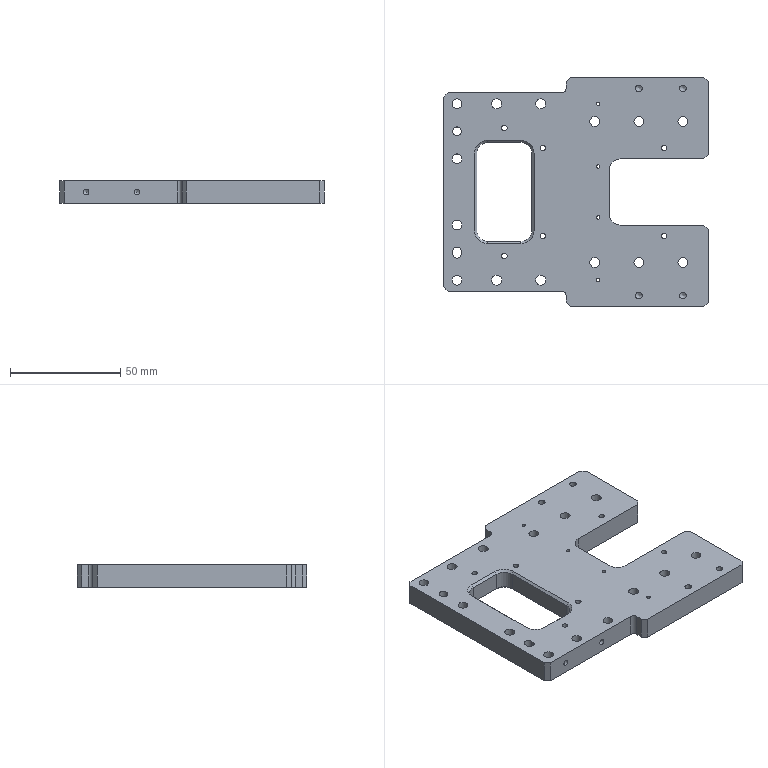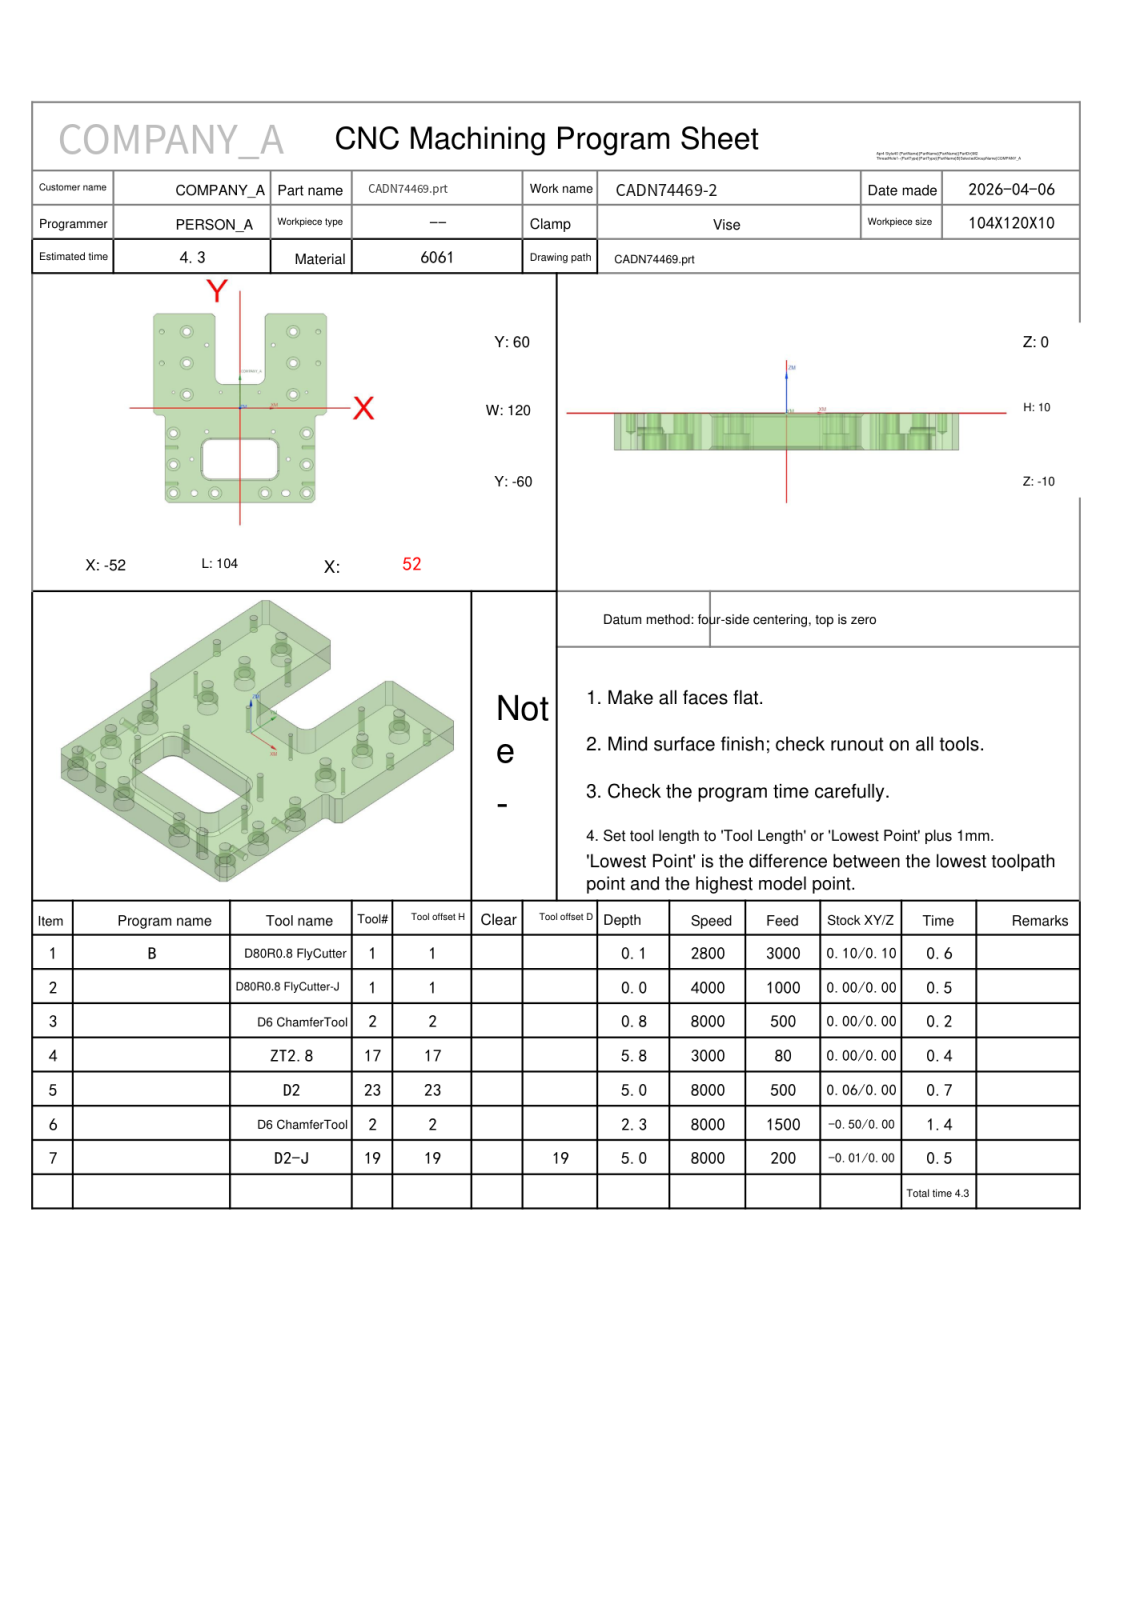NC program | NX | posted by the shop | part box 120 x 104 x 10 mm
Whole program:
%
O0001
(Machine time: 5.52 MIN)
(===Total Tool:5===)
(T1=D80R0.8 FlyCutter D=80.  R=0.8  D-  H01 Z=0.    )
(T2=D6 ChamferTool   D=6.   R=0.   D-  H02 Z=-2.3  )
(T17=ZT2.8  D=2.8  DR_a=118 D-  H17 Z=-5.8  )
(T23=D2     D=2.   R=0.   D-  H23 Z=-5.   )
(T19=D2-J   D=2.   R=0.   D19 H19 Z=-5.   )
G80 G90 G17 G49 G40
G91 G28 Z0
M01
N1 T01 M06
(D80R0.8 FlyCutter  D=80. R=0.8 H=01 ce=0.10 di=0.10)
G00 G90 G54 X-28.097 Y-112.097 M03 S2800
G43 H01 Z20.
M08
Z3.525
G01 Z1.525 F3000.
Y-100.097
Y92.1
G02 X-20.099 Y100.097 I8. J-.003
G01 X12.737
G02 X20.737 Y92.097 I0.0 J-8.
G01 Y-100.097
Y-112.097
Z3.525
G00 X-28.097
Z3.05
G01 Z1.05
Y-100.097
Y92.1
G02 X-20.099 Y100.097 I8. J-.003
G01 X12.737
G02 X20.737 Y92.097 I0.0 J-8.
G01 Y-100.097
Y-112.097
Z3.05
G00 X-28.097
Z2.575
G01 Z.575
Y-100.097
Y92.1
G02 X-20.099 Y100.097 I8. J-.003
G01 X12.737
G02 X20.737 Y92.097 I0.0 J-8.
G01 Y-100.097
Y-112.097
Z2.575
G00 X-28.097
Z2.1
G01 Z.1
Y-100.097
Y92.1
G02 X-20.099 Y100.097 I8. J-.003
G01 X12.737
G02 X20.737 Y92.097 I0.0 J-8.
G01 Y-100.097
Y-112.097
Z2.1
G00 Z20.
G91 G28 Z0.0
M05
M09
G91 G28 Z0.0
M01
N2 T01 M06
(D80R0.8 FlyCutter-J  D=80. R=0.8 H=01 ce=0.00 di=0.00)
G00 G90 G54 X-27.999 Y-111.999 M03 S4000
G43 H01 Z20.
M08
Z2.
G01 Z0.0 F1000.
Y-99.999
Y92.002
G02 X-20.002 Y99.999 I8. J-.003
G01 X12.639
G02 X20.639 Y91.999 I0.0 J-8.
G01 Y-99.999
Y-111.999
Z2.
G00 Z20.
G91 G28 Z0.0
M05
M09
G91 G28 Z0.0
M01
N3 T02 M06
(D6 ChamferTool  D=6. R=0. H=02 ce=0.00 di=0.00)
G00 G90 G54 X47. Y48.5 M03 S8000
G43 H02 Z20.
M08
G98 G81 X47. Y48.5 Z-.8 R1. F500.
X32.
X20. Y40.
X32. Y28.5
X47.
X40. Y10.
X32. Y8.5
X11.54 Y10.
X20. Y-15.
X40. Y-16.
X29. Y-32.5
X40. Y-36.
Y-54.
X15.
X-15.
X-27.5
X-40.
Y-36.
X-29. Y-32.5
X-40. Y-16.
X-20. Y-15.
X-11.54 Y10.
X-32. Y8.5
X-40. Y10.
X-47. Y28.5
X-32.
X-20. Y40.
X-32. Y48.5
X-47.
G80
G00 Z20.
G91 G28 Z0.0
M05
M09
G91 G28 Z0.0
M01
N4 T17 M06
(ZT2.8 D=2.8 DR_a=118 H=17)
G00 G90 G54 X47. Y28.5 M03 S3000
G43 H17 Z20.
M08
G98 G83 X47. Y28.5 Z-5.801 R1. F80. Q3.
Y48.5
X-47.
Y28.5
G80
G00 Z20.
G91 G28 Z0.0
M05
M09
G91 G28 Z0.0
M01
N5 T23 M06
(D2  D=2. R=0. H=23 ce=0.06 di=0.00)
G00 G90 G54 X47. Y28.5 M03 S8000
G43 H23 Z20.
M08
Z.5
G03 X47.22 Y28.72 I0.0 J.22 F500.
X47. Y28.94 I-.22 J0.0
X47. Y28.94 Z.3 I0.0 J-.44
X47. Y28.94 Z.1 I0.0 J-.44
X47. Y28.94 Z-.1 I0.0 J-.44
X47. Y28.94 Z-.3 I0.0 J-.44
X47. Y28.94 Z-.5 I0.0 J-.44
X47. Y28.94 Z-.7 I0.0 J-.44
X47. Y28.94 Z-.9 I0.0 J-.44
X47. Y28.94 Z-1.1 I0.0 J-.44
X47. Y28.94 Z-1.3 I0.0 J-.44
X47. Y28.94 Z-1.5 I0.0 J-.44
X47. Y28.94 Z-1.7 I0.0 J-.44
X47. Y28.94 Z-1.9 I0.0 J-.44
X47. Y28.94 Z-2.1 I0.0 J-.44
X47. Y28.94 Z-2.3 I0.0 J-.44
X47. Y28.94 Z-2.5 I0.0 J-.44
X47. Y28.94 Z-2.7 I0.0 J-.44
X47. Y28.94 Z-2.9 I0.0 J-.44
X47. Y28.94 Z-3.1 I0.0 J-.44
X47. Y28.94 Z-3.3 I0.0 J-.44
X47. Y28.94 Z-3.5 I0.0 J-.44
X47. Y28.94 Z-3.7 I0.0 J-.44
X47. Y28.94 Z-3.9 I0.0 J-.44
X47. Y28.94 Z-4.1 I0.0 J-.44
X47. Y28.94 Z-4.3 I0.0 J-.44
X47. Y28.94 Z-4.5 I0.0 J-.44
X47. Y28.94 Z-4.7 I0.0 J-.44
X47. Y28.94 Z-4.9 I0.0 J-.44
X47. Y28.06 Z-5. I0.0 J-.44
X47.44 Y28.5 I0.0 J.44
X47. Y28.94 I-.44 J0.0
X46.56 Y28.5 I0.0 J-.44
X47. Y28.06 I.44 J0.0
X47.22 Y28.28 I0.0 J.22
X47. Y28.5 I-.22 J0.0
G00 Z20.
Y48.5
Z.5
G03 X47.22 Y48.72 I0.0 J.22
X47. Y48.94 I-.22 J0.0
X47. Y48.94 Z.3 I0.0 J-.44
X47. Y48.94 Z.1 I0.0 J-.44
X47. Y48.94 Z-.1 I0.0 J-.44
X47. Y48.94 Z-.3 I0.0 J-.44
X47. Y48.94 Z-.5 I0.0 J-.44
X47. Y48.94 Z-.7 I0.0 J-.44
X47. Y48.94 Z-.9 I0.0 J-.44
X47. Y48.94 Z-1.1 I0.0 J-.44
X47. Y48.94 Z-1.3 I0.0 J-.44
X47. Y48.94 Z-1.5 I0.0 J-.44
X47. Y48.94 Z-1.7 I0.0 J-.44
X47. Y48.94 Z-1.9 I0.0 J-.44
X47. Y48.94 Z-2.1 I0.0 J-.44
X47. Y48.94 Z-2.3 I0.0 J-.44
X47. Y48.94 Z-2.5 I0.0 J-.44
X47. Y48.94 Z-2.7 I0.0 J-.44
X47. Y48.94 Z-2.9 I0.0 J-.44
X47. Y48.94 Z-3.1 I0.0 J-.44
X47. Y48.94 Z-3.3 I0.0 J-.44
X47. Y48.94 Z-3.5 I0.0 J-.44
X47. Y48.94 Z-3.7 I0.0 J-.44
X47. Y48.94 Z-3.9 I0.0 J-.44
X47. Y48.94 Z-4.1 I0.0 J-.44
X47. Y48.94 Z-4.3 I0.0 J-.44
X47. Y48.94 Z-4.5 I0.0 J-.44
X47. Y48.94 Z-4.7 I0.0 J-.44
X47. Y48.94 Z-4.9 I0.0 J-.44
X47. Y48.06 Z-5. I0.0 J-.44
X47.44 Y48.5 I0.0 J.44
X47. Y48.94 I-.44 J0.0
X46.56 Y48.5 I0.0 J-.44
X47. Y48.06 I.44 J0.0
X47.22 Y48.28 I0.0 J.22
X47. Y48.5 I-.22 J0.0
G00 Z20.
X-47.
Z.5
G03 X-46.78 Y48.72 I0.0 J.22
X-47. Y48.94 I-.22 J0.0
X-47. Y48.94 Z.3 I0.0 J-.44
X-47. Y48.94 Z.1 I0.0 J-.44
X-47. Y48.94 Z-.1 I0.0 J-.44
X-47. Y48.94 Z-.3 I0.0 J-.44
X-47. Y48.94 Z-.5 I0.0 J-.44
X-47. Y48.94 Z-.7 I0.0 J-.44
X-47. Y48.94 Z-.9 I0.0 J-.44
X-47. Y48.94 Z-1.1 I0.0 J-.44
X-47. Y48.94 Z-1.3 I0.0 J-.44
X-47. Y48.94 Z-1.5 I0.0 J-.44
X-47. Y48.94 Z-1.7 I0.0 J-.44
X-47. Y48.94 Z-1.9 I0.0 J-.44
X-47. Y48.94 Z-2.1 I0.0 J-.44
X-47. Y48.94 Z-2.3 I0.0 J-.44
X-47. Y48.94 Z-2.5 I0.0 J-.44
X-47. Y48.94 Z-2.7 I0.0 J-.44
X-47. Y48.94 Z-2.9 I0.0 J-.44
X-47. Y48.94 Z-3.1 I0.0 J-.44
X-47. Y48.94 Z-3.3 I0.0 J-.44
X-47. Y48.94 Z-3.5 I0.0 J-.44
X-47. Y48.94 Z-3.7 I0.0 J-.44
X-47. Y48.94 Z-3.9 I0.0 J-.44
X-47. Y48.94 Z-4.1 I0.0 J-.44
X-47. Y48.94 Z-4.3 I0.0 J-.44
X-47. Y48.94 Z-4.5 I0.0 J-.44
X-47. Y48.94 Z-4.7 I0.0 J-.44
X-47. Y48.94 Z-4.9 I0.0 J-.44
X-47. Y48.06 Z-5. I0.0 J-.44
X-46.56 Y48.5 I0.0 J.44
X-47. Y48.94 I-.44 J0.0
X-47.44 Y48.5 I0.0 J-.44
X-47. Y48.06 I.44 J0.0
X-46.78 Y48.28 I0.0 J.22
X-47. Y48.5 I-.22 J0.0
G00 Z20.
Y28.5
Z.5
G03 X-46.78 Y28.72 I0.0 J.22
X-47. Y28.94 I-.22 J0.0
X-47. Y28.94 Z.3 I0.0 J-.44
X-47. Y28.94 Z.1 I0.0 J-.44
X-47. Y28.94 Z-.1 I0.0 J-.44
X-47. Y28.94 Z-.3 I0.0 J-.44
X-47. Y28.94 Z-.5 I0.0 J-.44
X-47. Y28.94 Z-.7 I0.0 J-.44
X-47. Y28.94 Z-.9 I0.0 J-.44
X-47. Y28.94 Z-1.1 I0.0 J-.44
X-47. Y28.94 Z-1.3 I0.0 J-.44
X-47. Y28.94 Z-1.5 I0.0 J-.44
X-47. Y28.94 Z-1.7 I0.0 J-.44
X-47. Y28.94 Z-1.9 I0.0 J-.44
X-47. Y28.94 Z-2.1 I0.0 J-.44
X-47. Y28.94 Z-2.3 I0.0 J-.44
X-47. Y28.94 Z-2.5 I0.0 J-.44
X-47. Y28.94 Z-2.7 I0.0 J-.44
X-47. Y28.94 Z-2.9 I0.0 J-.44
X-47. Y28.94 Z-3.1 I0.0 J-.44
X-47. Y28.94 Z-3.3 I0.0 J-.44
X-47. Y28.94 Z-3.5 I0.0 J-.44
X-47. Y28.94 Z-3.7 I0.0 J-.44
X-47. Y28.94 Z-3.9 I0.0 J-.44
X-47. Y28.94 Z-4.1 I0.0 J-.44
X-47. Y28.94 Z-4.3 I0.0 J-.44
X-47. Y28.94 Z-4.5 I0.0 J-.44
X-47. Y28.94 Z-4.7 I0.0 J-.44
X-47. Y28.94 Z-4.9 I0.0 J-.44
X-47. Y28.06 Z-5. I0.0 J-.44
X-46.56 Y28.5 I0.0 J.44
X-47. Y28.94 I-.44 J0.0
X-47.44 Y28.5 I0.0 J-.44
X-47. Y28.06 I.44 J0.0
X-46.78 Y28.28 I0.0 J.22
X-47. Y28.5 I-.22 J0.0
G00 Z20.
G91 G28 Z0.0
M05
M09
G91 G28 Z0.0
M01
N6 T02 M06
(D6 ChamferTool  D=6. R=0. H=02 ce=-0.50 di=0.00)
G00 G90 G54 X7.884 Y-44.5 M03 S7000
G43 H02 Z20.
M08
Z2.5
G01 X17.5 Z-1. F1500.
G03 X22. Y-40. I0.0 J4.5
G01 Y-25.
G03 X17.5 Y-20.5 I-4.5 J0.0
G01 X-17.5
G03 X-22. Y-25. I0.0 J-4.5
G01 Y-40.
G03 X-17.5 Y-44.5 I4.5 J0.0
G01 X17.5
G03 X17.999 Y-44.472 I0.0 J4.5
G01 Z1.5
G00 Z20.
G00 G90 X40. Y10. M03 S8000
Z20.
G98 G81 X40. Y10. Z-1.2 R3. F500.
X11.54
X-11.54
X-40.
G80
G00 Z20.
G00 G90 X20. Y40. M03 S8000
Z20.
G98 G81 X20. Y40. Z-1.75 R3. F500.
X-20.
Y-15.
X-29. Y-32.5
X20. Y-15.
X29. Y-32.5
G80
G00 Z20.
G00 G90 X47. Y28.5 M03 S8000
Z20.
G98 G81 X47. Y28.5 Z-1.8 R3. F500.
Y48.5
X-47.
Y28.5
G80
G00 Z20.
G00 G90 X-27.5 Y-54. M03 S8000
Z20.
G98 G81 X-27.5 Y-54. Z-2.3 R3. F500.
G80
G00 Z20.
G00 G90 X32.55 Y48.518 M03 S8000
Z20.
Z-.5
G01 Z-1. F500.
X33.5 Y48.55
G03 X32. Y50.05 I-1.5 J0.0
X30.45 Y48.5 I0.0 J-1.55
X32. Y46.95 I1.55 J0.0
X33.55 Y48.5 I0.0 J1.55
X32. Y50.05 I-1.55 J0.0
X30.5 Y48.55 I0.0 J-1.5
G01 X31.45 Y48.518
Z-.5
G00 Z20.
X32.55 Y28.518
Z-.5
G01 Z-1.
X33.5 Y28.55
G03 X32. Y30.05 I-1.5 J0.0
X30.45 Y28.5 I0.0 J-1.55
X32. Y26.95 I1.55 J0.0
X33.55 Y28.5 I0.0 J1.55
X32. Y30.05 I-1.55 J0.0
X30.5 Y28.55 I0.0 J-1.5
G01 X31.45 Y28.518
Z-.5
G00 Z20.
X32.55 Y8.518
Z-.5
G01 Z-1.
X33.5 Y8.55
G03 X32. Y10.05 I-1.5 J0.0
X30.45 Y8.5 I0.0 J-1.55
X32. Y6.95 I1.55 J0.0
X33.55 Y8.5 I0.0 J1.55
X32. Y10.05 I-1.55 J0.0
X30.5 Y8.55 I0.0 J-1.5
G01 X31.45 Y8.518
Z-.5
G00 Z20.
X40.55 Y-15.982
Z-.5
G01 Z-1.
X41.5 Y-15.95
G03 X40. Y-14.45 I-1.5 J0.0
X38.45 Y-16. I0.0 J-1.55
X40. Y-17.55 I1.55 J0.0
X41.55 Y-16. I0.0 J1.55
X40. Y-14.45 I-1.55 J0.0
X38.5 Y-15.95 I0.0 J-1.5
G01 X39.45 Y-15.982
Z-.5
G00 Z20.
X40.55 Y-35.982
Z-.5
G01 Z-1.
X41.5 Y-35.95
G03 X40. Y-34.45 I-1.5 J0.0
X38.45 Y-36. I0.0 J-1.55
X40. Y-37.55 I1.55 J0.0
X41.55 Y-36. I0.0 J1.55
X40. Y-34.45 I-1.55 J0.0
X38.5 Y-35.95 I0.0 J-1.5
G01 X39.45 Y-35.982
Z-.5
G00 Z20.
X40.55 Y-53.982
Z-.5
G01 Z-1.
X41.5 Y-53.95
G03 X40. Y-52.45 I-1.5 J0.0
X38.45 Y-54. I0.0 J-1.55
X40. Y-55.55 I1.55 J0.0
X41.55 Y-54. I0.0 J1.55
X40. Y-52.45 I-1.55 J0.0
X38.5 Y-53.95 I0.0 J-1.5
G01 X39.45 Y-53.982
Z-.5
G00 Z20.
X15.55
Z-.5
G01 Z-1.
X16.5 Y-53.95
G03 X15. Y-52.45 I-1.5 J0.0
X13.45 Y-54. I0.0 J-1.55
X15. Y-55.55 I1.55 J0.0
X16.55 Y-54. I0.0 J1.55
X15. Y-52.45 I-1.55 J0.0
X13.5 Y-53.95 I0.0 J-1.5
G01 X14.45 Y-53.982
Z-.5
G00 Z20.
X-14.45
Z-.5
G01 Z-1.
X-13.5 Y-53.95
G03 X-15. Y-52.45 I-1.5 J0.0
X-16.55 Y-54. I0.0 J-1.55
X-15. Y-55.55 I1.55 J0.0
X-13.45 Y-54. I0.0 J1.55
X-15. Y-52.45 I-1.55 J0.0
X-16.5 Y-53.95 I0.0 J-1.5
G01 X-15.55 Y-53.982
Z-.5
G00 Z20.
X-39.45
Z-.5
G01 Z-1.
X-38.5 Y-53.95
G03 X-40. Y-52.45 I-1.5 J0.0
X-41.55 Y-54. I0.0 J-1.55
X-40. Y-55.55 I1.55 J0.0
X-38.45 Y-54. I0.0 J1.55
X-40. Y-52.45 I-1.55 J0.0
X-41.5 Y-53.95 I0.0 J-1.5
G01 X-40.55 Y-53.982
Z-.5
G00 Z20.
X-39.45 Y-35.982
Z-.5
G01 Z-1.
X-38.5 Y-35.95
G03 X-40. Y-34.45 I-1.5 J0.0
X-41.55 Y-36. I0.0 J-1.55
X-40. Y-37.55 I1.55 J0.0
X-38.45 Y-36. I0.0 J1.55
X-40. Y-34.45 I-1.55 J0.0
X-41.5 Y-35.95 I0.0 J-1.5
G01 X-40.55 Y-35.982
Z-.5
G00 Z20.
X-39.45 Y-15.982
Z-.5
G01 Z-1.
X-38.5 Y-15.95
G03 X-40. Y-14.45 I-1.5 J0.0
X-41.55 Y-16. I0.0 J-1.55
X-40. Y-17.55 I1.55 J0.0
X-38.45 Y-16. I0.0 J1.55
X-40. Y-14.45 I-1.55 J0.0
X-41.5 Y-15.95 I0.0 J-1.5
G01 X-40.55 Y-15.982
Z-.5
G00 Z20.
X-31.45 Y8.518
Z-.5
G01 Z-1.
X-30.5 Y8.55
G03 X-32. Y10.05 I-1.5 J0.0
X-33.55 Y8.5 I0.0 J-1.55
X-32. Y6.95 I1.55 J0.0
X-30.45 Y8.5 I0.0 J1.55
X-32. Y10.05 I-1.55 J0.0
X-33.5 Y8.55 I0.0 J-1.5
G01 X-32.55 Y8.518
Z-.5
G00 Z20.
X-31.45 Y28.518
Z-.5
G01 Z-1.
X-30.5 Y28.55
G03 X-32. Y30.05 I-1.5 J0.0
X-33.55 Y28.5 I0.0 J-1.55
X-32. Y26.95 I1.55 J0.0
X-30.45 Y28.5 I0.0 J1.55
X-32. Y30.05 I-1.55 J0.0
X-33.5 Y28.55 I0.0 J-1.5
G01 X-32.55 Y28.518
Z-.5
G00 Z20.
X-31.45 Y48.518
Z-.5
G01 Z-1.
X-30.5 Y48.55
G03 X-32. Y50.05 I-1.5 J0.0
X-33.55 Y48.5 I0.0 J-1.55
X-32. Y46.95 I1.55 J0.0
X-30.45 Y48.5 I0.0 J1.55
X-32. Y50.05 I-1.55 J0.0
X-33.5 Y48.55 I0.0 J-1.5
G01 X-32.55 Y48.518
Z-.5
G00 Z20.
G00 G90 X41.046 Y60.7 M03 S7000
Z20.
Z2.5
G01 X49.953 Z-.742 F1500.
X50.16 Y60.662 Z-.819
X50.355 Y60.581 Z-.895
X50.528 Y60.462 Z-.972
X50.583 Y60.407 Z-1.
X52.407 Y58.583
G02 X52.7 Y57.876 I-.707 J-.707
G01 Y-2.376
G02 X52.407 Y-3.083 I-1. J0.0
G01 X50.583 Y-4.907
G02 X49.876 Y-5.2 I-.707 J.707
G01 X47.
G03 X45.7 Y-6.5 I0.0 J-1.3
G01 Y-57.876
G02 X45.407 Y-58.583 I-1. J0.0
G01 X43.583 Y-60.407
G02 X42.876 Y-60.7 I-.707 J.707
G01 X-42.876
G02 X-43.583 Y-60.407 I0.0 J1.
G01 X-45.407 Y-58.583
G02 X-45.7 Y-57.876 I.707 J.707
G01 Y-6.5
G03 X-47. Y-5.2 I-1.3 J0.0
G01 X-49.876
G02 X-50.583 Y-4.907 I0.0 J1.
G01 X-52.407 Y-3.083
G02 X-52.7 Y-2.376 I.707 J.707
G01 Y57.876
G02 X-52.407 Y58.583 I1. J0.0
G01 X-50.583 Y60.407
G02 X-49.876 Y60.7 I.707 J-.707
G01 X-17.124
G02 X-16.417 Y60.407 I0.0 J-1.
G01 X-14.593 Y58.583
G02 X-14.3 Y57.876 I-.707 J-.707
G01 Y20.
G03 X-10. Y15.7 I4.3 J0.0
G01 X10.
G03 X14.3 Y20. I0.0 J4.3
G01 Y57.876
G02 X14.593 Y58.583 I1. J0.0
G01 X16.417 Y60.407
G02 X17.124 Y60.7 I.707 J-.707
G01 X49.876
G02 X50.583 Y60.407 I0.0 J-1.
G01 X50.936 Y60.054
Z1.5
G00 Z20.
X27.56 Y-55.3
Z2.5
G01 X28.088 Z2.308
X28.319 Y-55.263 Z2.223
X28.539 Y-55.186 Z2.138
X28.742 Y-55.071 Z2.053
X28.921 Y-54.921 Z1.968
X29.071 Y-54.742 Z1.883
X29.186 Y-54.539 Z1.798
X29.263 Y-54.319 Z1.713
X29.3 Y-54.088 Z1.628
Y-53.912 Z1.564
X29.263 Y-53.681 Z1.479
X29.186 Y-53.461 Z1.394
X29.071 Y-53.258 Z1.309
X28.921 Y-53.079 Z1.224
X28.742 Y-52.929 Z1.139
X28.539 Y-52.814 Z1.054
X28.319 Y-52.737 Z.969
X28.088 Y-52.7 Z.884
X26.912 Z.456
X26.681 Y-52.737 Z.371
X26.461 Y-52.814 Z.286
X26.258 Y-52.929 Z.201
X26.079 Y-53.079 Z.116
X25.929 Y-53.258 Z.031
X25.814 Y-53.461 Z-.054
X25.737 Y-53.681 Z-.139
X25.7 Y-53.912 Z-.224
Y-54.088 Z-.288
X25.737 Y-54.319 Z-.373
X25.814 Y-54.539 Z-.458
X25.929 Y-54.742 Z-.543
X26.079 Y-54.921 Z-.628
X26.258 Y-55.071 Z-.713
X26.461 Y-55.186 Z-.798
X26.681 Y-55.263 Z-.883
X26.912 Y-55.3 Z-.968
X27. Z-1.
X28.
G03 X29.3 Y-54. I0.0 J1.3
X28. Y-52.7 I-1.3 J0.0
G01 X27.
G03 X25.7 Y-54. I0.0 J-1.3
X27. Y-55.3 I1.3 J0.0
G01 X27.5
Z1.5
G00 Z20.
G00 G90 X-18.7 Y-42.858 M03 S6500
Z20.
Z-.2
G01 Z-1.7 F1500.
Y-43.1
G03 X-17.5 Y-44.3 I1.2 J0.0
G01 X17.5
G03 X21.8 Y-40. I0.0 J4.3
G01 Y-25.
G03 X17.5 Y-20.7 I-4.3 J0.0
G01 X-17.5
G03 X-17.89 Y-20.718 I0.0 J-4.3
X-18.179 Y-20.754 I.39 J-4.282
G01 X-18.22 Y-20.761
G03 X-21.783 Y-24.621 I.72 J-4.239
G01 X-21.786 Y-24.659
X-21.794 Y-24.768
X-21.797 Y-24.83
X-21.798 Y-24.885
X-21.8 Y-25.
Y-40.
G03 X-17.5 Y-44.3 I4.3 J0.0
G01 X-17.1
G03 X-15.9 Y-43.1 I0.0 J1.2
G01 Z-.2
G00 Z20.
G91 G28 Z0.0
M05
M09
G91 G28 Z0.0
M01
N7 T19 M06
(D2-J  D=2. R=0. H=19 ce=-0.01 di=0.00)
G00 G90 G54 X47. Y28.5 M03 S8000
G43 H19 Z20.
M08
Z.5
G41 D19
G01 X47.147 Y28.636 F200.
X47.216 Y28.794
G03 X47. Y29.01 I-.216 J0.0
X47. Y29.01 Z-.5 I0.0 J-.51
X47. Y29.01 Z-1.5 I0.0 J-.51
X47. Y29.01 Z-2.5 I0.0 J-.51
X47. Y29.01 Z-3.5 I0.0 J-.51
X47. Y29.01 Z-4.5 I0.0 J-.51
X47. Y27.99 Z-5. I0.0 J-.51
X47.51 Y28.5 I0.0 J.51
X47. Y29.01 I-.51 J0.0
X46.49 Y28.5 I0.0 J-.51
X47. Y27.99 I.51 J0.0
X47.216 Y28.206 I0.0 J.216
G01 X47.147 Y28.364
G40 X47. Y28.5
G00 Z20.
Y48.5
Z.5
G41 D19
G01 X47.147 Y48.636
X47.216 Y48.794
G03 X47. Y49.01 I-.216 J0.0
X47. Y49.01 Z-.5 I0.0 J-.51
X47. Y49.01 Z-1.5 I0.0 J-.51
X47. Y49.01 Z-2.5 I0.0 J-.51
X47. Y49.01 Z-3.5 I0.0 J-.51
X47. Y49.01 Z-4.5 I0.0 J-.51
X47. Y47.99 Z-5. I0.0 J-.51
X47.51 Y48.5 I0.0 J.51
X47. Y49.01 I-.51 J0.0
X46.49 Y48.5 I0.0 J-.51
X47. Y47.99 I.51 J0.0
X47.216 Y48.206 I0.0 J.216
G01 X47.147 Y48.364
G40 X47. Y48.5
G00 Z20.
X-47.
Z.5
G41 D19
G01 X-46.853 Y48.636
X-46.784 Y48.794
G03 X-47. Y49.01 I-.216 J0.0
X-47. Y49.01 Z-.5 I0.0 J-.51
X-47. Y49.01 Z-1.5 I0.0 J-.51
X-47. Y49.01 Z-2.5 I0.0 J-.51
X-47. Y49.01 Z-3.5 I0.0 J-.51
X-47. Y49.01 Z-4.5 I0.0 J-.51
X-47. Y47.99 Z-5. I0.0 J-.51
X-46.49 Y48.5 I0.0 J.51
X-47. Y49.01 I-.51 J0.0
X-47.51 Y48.5 I0.0 J-.51
X-47. Y47.99 I.51 J0.0
X-46.784 Y48.206 I0.0 J.216
G01 X-46.853 Y48.364
G40 X-47. Y48.5
G00 Z20.
Y28.5
Z.5
G41 D19
G01 X-46.853 Y28.636
X-46.784 Y28.794
G03 X-47. Y29.01 I-.216 J0.0
X-47. Y29.01 Z-.5 I0.0 J-.51
X-47. Y29.01 Z-1.5 I0.0 J-.51
X-47. Y29.01 Z-2.5 I0.0 J-.51
X-47. Y29.01 Z-3.5 I0.0 J-.51
X-47. Y29.01 Z-4.5 I0.0 J-.51
X-47. Y27.99 Z-5. I0.0 J-.51
X-46.49 Y28.5 I0.0 J.51
X-47. Y29.01 I-.51 J0.0
X-47.51 Y28.5 I0.0 J-.51
X-47. Y27.99 I.51 J0.0
X-46.784 Y28.206 I0.0 J.216
G01 X-46.853 Y28.364
G40 X-47. Y28.5
G00 Z20.
M05
M09
G91 G28 Z0.0
G91 G28 Y0.0
M30
%